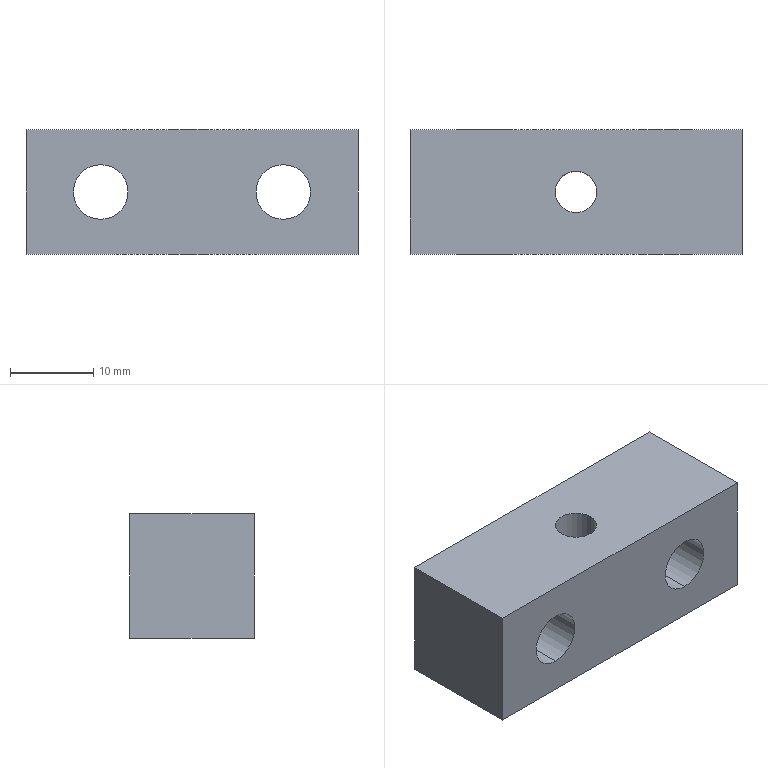Part | STEP file | 0243_214_Block | 1 solid | 12 faces | box 40 x 15 x 15 mm | volume 7679 mm3 | cylinder 6 | plane 6 | commonest cylinder face diameters 6.6 x4 5 x2
STEP:
#1=CARTESIAN_POINT('',(0.,0.,0.));
#2=DIRECTION('',(0.,0.,1.));
#3=DIRECTION('',(1.,0.,0.));
#4=AXIS2_PLACEMENT_3D('',#1,#2,#3);
#5=CARTESIAN_POINT('',(11.,0.,-4.2));
#6=VERTEX_POINT('',#5);
#7=CARTESIAN_POINT('',(11.,15.,-4.2));
#8=VERTEX_POINT('',#7);
#9=CARTESIAN_POINT('',(11.,15.,-4.2));
#10=DIRECTION('',(0.,1.,0.));
#11=VECTOR('',#10,1.);
#12=LINE('',#9,#11);
#13=CARTESIAN_POINT('',(11.,15.,-7.5));
#14=DIRECTION('',(0.,1.,0.));
#15=DIRECTION('',(0.,0.,1.));
#16=AXIS2_PLACEMENT_3D('',#13,#14,#15);
#17=CYLINDRICAL_SURFACE('',#16,3.3);
#18=CARTESIAN_POINT('',(6.283,0.));
#19=DIRECTION('',(0.,1.));
#20=VECTOR('',#19,1.);
#21=LINE('',#18,#20);
#22=(GEOMETRIC_REPRESENTATION_CONTEXT(2)PARAMETRIC_REPRESENTATION_CONTEXT()REPRESENTATION_CONTEXT('',''));
#23=DEFINITIONAL_REPRESENTATION('',(#21),#22);
#24=PCURVE('',#17,#23);
#25=CARTESIAN_POINT('',(11.,15.,-7.5));
#26=DIRECTION('',(0.,1.,0.));
#27=DIRECTION('',(0.,0.,1.));
#28=AXIS2_PLACEMENT_3D('',#25,#26,#27);
#29=CYLINDRICAL_SURFACE('',#28,3.3);
#30=CARTESIAN_POINT('',(0.,0.));
#31=DIRECTION('',(0.,1.));
#32=VECTOR('',#31,1.);
#33=LINE('',#30,#32);
#34=(GEOMETRIC_REPRESENTATION_CONTEXT(2)PARAMETRIC_REPRESENTATION_CONTEXT()REPRESENTATION_CONTEXT('',''));
#35=DEFINITIONAL_REPRESENTATION('',(#33),#34);
#36=PCURVE('',#29,#35);
#37=SURFACE_CURVE('',#12,(#24,#36),.PCURVE_S1.);
#38=EDGE_CURVE('',#6,#8,#37,.T.);
#39=ORIENTED_EDGE('',*,*,#38,.T.);
#40=CARTESIAN_POINT('',(11.,15.,-10.8));
#41=VERTEX_POINT('',#40);
#42=CARTESIAN_POINT('',(11.,15.,-7.5));
#43=DIRECTION('',(0.,1.,0.));
#44=DIRECTION('',(0.,0.,1.));
#45=AXIS2_PLACEMENT_3D('',#42,#43,#44);
#46=CIRCLE('',#45,3.3);
#47=CARTESIAN_POINT('',(0.,0.));
#48=DIRECTION('',(1.,0.));
#49=VECTOR('',#48,1.);
#50=LINE('',#47,#49);
#51=(GEOMETRIC_REPRESENTATION_CONTEXT(2)PARAMETRIC_REPRESENTATION_CONTEXT()REPRESENTATION_CONTEXT('',''));
#52=DEFINITIONAL_REPRESENTATION('',(#50),#51);
#53=PCURVE('',#17,#52);
#54=CARTESIAN_POINT('',(-20.,15.,-15.));
#55=DIRECTION('',(0.,-1.,0.));
#56=DIRECTION('',(0.,0.,-1.));
#57=AXIS2_PLACEMENT_3D('',#54,#55,#56);
#58=PLANE('',#57);
#59=CARTESIAN_POINT('',(-10.8,31.));
#60=CARTESIAN_POINT('',(-10.8,36.716));
#61=CARTESIAN_POINT('',(-5.85,33.858));
#62=CARTESIAN_POINT('',(-0.9,31.));
#63=CARTESIAN_POINT('',(-5.85,28.142));
#64=CARTESIAN_POINT('',(-10.8,25.284));
#65=CARTESIAN_POINT('',(-10.8,31.));
#66=(BOUNDED_CURVE()B_SPLINE_CURVE(2,(#59,#60,#61,#62,#63,#64,#65),.UNSPECIFIED.,.T.,.F.)B_SPLINE_CURVE_WITH_KNOTS((1,2,2,2,2,1),(-2.094,0.,2.094,4.189,6.283,8.378),.UNSPECIFIED.)CURVE()GEOMETRIC_REPRESENTATION_ITEM()RATIONAL_B_SPLINE_CURVE((1.,0.5,1.,0.5,1.,0.5,1.))REPRESENTATION_ITEM(''));
#67=(GEOMETRIC_REPRESENTATION_CONTEXT(2)PARAMETRIC_REPRESENTATION_CONTEXT()REPRESENTATION_CONTEXT('',''));
#68=DEFINITIONAL_REPRESENTATION('',(#66),#67);
#69=PCURVE('',#58,#68);
#70=SURFACE_CURVE('',#46,(#53,#69),.PCURVE_S1.);
#71=EDGE_CURVE('',#41,#8,#70,.T.);
#72=ORIENTED_EDGE('',*,*,#71,.F.);
#73=CARTESIAN_POINT('',(11.,0.,-10.8));
#74=VERTEX_POINT('',#73);
#75=CARTESIAN_POINT('',(11.,15.,-10.8));
#76=DIRECTION('',(0.,1.,0.));
#77=VECTOR('',#76,1.);
#78=LINE('',#75,#77);
#79=CARTESIAN_POINT('',(3.142,0.));
#80=DIRECTION('',(0.,1.));
#81=VECTOR('',#80,1.);
#82=LINE('',#79,#81);
#83=(GEOMETRIC_REPRESENTATION_CONTEXT(2)PARAMETRIC_REPRESENTATION_CONTEXT()REPRESENTATION_CONTEXT('',''));
#84=DEFINITIONAL_REPRESENTATION('',(#82),#83);
#85=PCURVE('',#17,#84);
#86=CARTESIAN_POINT('',(3.142,0.));
#87=DIRECTION('',(0.,1.));
#88=VECTOR('',#87,1.);
#89=LINE('',#86,#88);
#90=(GEOMETRIC_REPRESENTATION_CONTEXT(2)PARAMETRIC_REPRESENTATION_CONTEXT()REPRESENTATION_CONTEXT('',''));
#91=DEFINITIONAL_REPRESENTATION('',(#89),#90);
#92=PCURVE('',#29,#91);
#93=SURFACE_CURVE('',#78,(#85,#92),.PCURVE_S1.);
#94=EDGE_CURVE('',#74,#41,#93,.T.);
#95=ORIENTED_EDGE('',*,*,#94,.F.);
#96=CARTESIAN_POINT('',(11.,0.,-7.5));
#97=DIRECTION('',(0.,1.,0.));
#98=DIRECTION('',(0.,0.,1.));
#99=AXIS2_PLACEMENT_3D('',#96,#97,#98);
#100=CIRCLE('',#99,3.3);
#101=CARTESIAN_POINT('',(0.,-15.));
#102=DIRECTION('',(1.,0.));
#103=VECTOR('',#102,1.);
#104=LINE('',#101,#103);
#105=(GEOMETRIC_REPRESENTATION_CONTEXT(2)PARAMETRIC_REPRESENTATION_CONTEXT()REPRESENTATION_CONTEXT('',''));
#106=DEFINITIONAL_REPRESENTATION('',(#104),#105);
#107=PCURVE('',#17,#106);
#108=CARTESIAN_POINT('',(-20.,0.,-15.));
#109=DIRECTION('',(0.,-1.,0.));
#110=DIRECTION('',(0.,0.,-1.));
#111=AXIS2_PLACEMENT_3D('',#108,#109,#110);
#112=PLANE('',#111);
#113=CARTESIAN_POINT('',(-10.8,31.));
#114=CARTESIAN_POINT('',(-10.8,36.716));
#115=CARTESIAN_POINT('',(-5.85,33.858));
#116=CARTESIAN_POINT('',(-0.9,31.));
#117=CARTESIAN_POINT('',(-5.85,28.142));
#118=CARTESIAN_POINT('',(-10.8,25.284));
#119=CARTESIAN_POINT('',(-10.8,31.));
#120=(BOUNDED_CURVE()B_SPLINE_CURVE(2,(#113,#114,#115,#116,#117,#118,#119),.UNSPECIFIED.,.T.,.F.)B_SPLINE_CURVE_WITH_KNOTS((1,2,2,2,2,1),(-2.094,0.,2.094,4.189,6.283,8.378),.UNSPECIFIED.)CURVE()GEOMETRIC_REPRESENTATION_ITEM()RATIONAL_B_SPLINE_CURVE((1.,0.5,1.,0.5,1.,0.5,1.))REPRESENTATION_ITEM(''));
#121=(GEOMETRIC_REPRESENTATION_CONTEXT(2)PARAMETRIC_REPRESENTATION_CONTEXT()REPRESENTATION_CONTEXT('',''));
#122=DEFINITIONAL_REPRESENTATION('',(#120),#121);
#123=PCURVE('',#112,#122);
#124=SURFACE_CURVE('',#100,(#107,#123),.PCURVE_S1.);
#125=EDGE_CURVE('',#74,#6,#124,.T.);
#126=ORIENTED_EDGE('',*,*,#125,.T.);
#127=EDGE_LOOP('',(#39,#72,#95,#126));
#128=FACE_BOUND('',#127,.F.);
#129=ADVANCED_FACE('',(#128),#17,.F.);
#130=CARTESIAN_POINT('',(-11.,0.,-4.2));
#131=VERTEX_POINT('',#130);
#132=CARTESIAN_POINT('',(-11.,15.,-4.2));
#133=VERTEX_POINT('',#132);
#134=CARTESIAN_POINT('',(-11.,15.,-4.2));
#135=DIRECTION('',(0.,1.,0.));
#136=VECTOR('',#135,1.);
#137=LINE('',#134,#136);
#138=CARTESIAN_POINT('',(-11.,15.,-7.5));
#139=DIRECTION('',(0.,1.,0.));
#140=DIRECTION('',(0.,0.,1.));
#141=AXIS2_PLACEMENT_3D('',#138,#139,#140);
#142=CYLINDRICAL_SURFACE('',#141,3.3);
#143=CARTESIAN_POINT('',(6.283,0.));
#144=DIRECTION('',(0.,1.));
#145=VECTOR('',#144,1.);
#146=LINE('',#143,#145);
#147=(GEOMETRIC_REPRESENTATION_CONTEXT(2)PARAMETRIC_REPRESENTATION_CONTEXT()REPRESENTATION_CONTEXT('',''));
#148=DEFINITIONAL_REPRESENTATION('',(#146),#147);
#149=PCURVE('',#142,#148);
#150=CARTESIAN_POINT('',(-11.,15.,-7.5));
#151=DIRECTION('',(0.,1.,0.));
#152=DIRECTION('',(0.,0.,1.));
#153=AXIS2_PLACEMENT_3D('',#150,#151,#152);
#154=CYLINDRICAL_SURFACE('',#153,3.3);
#155=CARTESIAN_POINT('',(0.,0.));
#156=DIRECTION('',(0.,1.));
#157=VECTOR('',#156,1.);
#158=LINE('',#155,#157);
#159=(GEOMETRIC_REPRESENTATION_CONTEXT(2)PARAMETRIC_REPRESENTATION_CONTEXT()REPRESENTATION_CONTEXT('',''));
#160=DEFINITIONAL_REPRESENTATION('',(#158),#159);
#161=PCURVE('',#154,#160);
#162=SURFACE_CURVE('',#137,(#149,#161),.PCURVE_S1.);
#163=EDGE_CURVE('',#131,#133,#162,.T.);
#164=ORIENTED_EDGE('',*,*,#163,.T.);
#165=CARTESIAN_POINT('',(-11.,15.,-10.8));
#166=VERTEX_POINT('',#165);
#167=CARTESIAN_POINT('',(-11.,15.,-7.5));
#168=DIRECTION('',(0.,1.,0.));
#169=DIRECTION('',(0.,0.,1.));
#170=AXIS2_PLACEMENT_3D('',#167,#168,#169);
#171=CIRCLE('',#170,3.3);
#172=CARTESIAN_POINT('',(0.,0.));
#173=DIRECTION('',(1.,0.));
#174=VECTOR('',#173,1.);
#175=LINE('',#172,#174);
#176=(GEOMETRIC_REPRESENTATION_CONTEXT(2)PARAMETRIC_REPRESENTATION_CONTEXT()REPRESENTATION_CONTEXT('',''));
#177=DEFINITIONAL_REPRESENTATION('',(#175),#176);
#178=PCURVE('',#142,#177);
#179=CARTESIAN_POINT('',(-10.8,9.));
#180=CARTESIAN_POINT('',(-10.8,14.716));
#181=CARTESIAN_POINT('',(-5.85,11.858));
#182=CARTESIAN_POINT('',(-0.9,9.));
#183=CARTESIAN_POINT('',(-5.85,6.142));
#184=CARTESIAN_POINT('',(-10.8,3.284));
#185=CARTESIAN_POINT('',(-10.8,9.));
#186=(BOUNDED_CURVE()B_SPLINE_CURVE(2,(#179,#180,#181,#182,#183,#184,#185),.UNSPECIFIED.,.T.,.F.)B_SPLINE_CURVE_WITH_KNOTS((1,2,2,2,2,1),(-2.094,0.,2.094,4.189,6.283,8.378),.UNSPECIFIED.)CURVE()GEOMETRIC_REPRESENTATION_ITEM()RATIONAL_B_SPLINE_CURVE((1.,0.5,1.,0.5,1.,0.5,1.))REPRESENTATION_ITEM(''));
#187=(GEOMETRIC_REPRESENTATION_CONTEXT(2)PARAMETRIC_REPRESENTATION_CONTEXT()REPRESENTATION_CONTEXT('',''));
#188=DEFINITIONAL_REPRESENTATION('',(#186),#187);
#189=PCURVE('',#58,#188);
#190=SURFACE_CURVE('',#171,(#178,#189),.PCURVE_S1.);
#191=EDGE_CURVE('',#166,#133,#190,.T.);
#192=ORIENTED_EDGE('',*,*,#191,.F.);
#193=CARTESIAN_POINT('',(-11.,0.,-10.8));
#194=VERTEX_POINT('',#193);
#195=CARTESIAN_POINT('',(-11.,15.,-10.8));
#196=DIRECTION('',(0.,1.,0.));
#197=VECTOR('',#196,1.);
#198=LINE('',#195,#197);
#199=CARTESIAN_POINT('',(3.142,0.));
#200=DIRECTION('',(0.,1.));
#201=VECTOR('',#200,1.);
#202=LINE('',#199,#201);
#203=(GEOMETRIC_REPRESENTATION_CONTEXT(2)PARAMETRIC_REPRESENTATION_CONTEXT()REPRESENTATION_CONTEXT('',''));
#204=DEFINITIONAL_REPRESENTATION('',(#202),#203);
#205=PCURVE('',#142,#204);
#206=CARTESIAN_POINT('',(3.142,0.));
#207=DIRECTION('',(0.,1.));
#208=VECTOR('',#207,1.);
#209=LINE('',#206,#208);
#210=(GEOMETRIC_REPRESENTATION_CONTEXT(2)PARAMETRIC_REPRESENTATION_CONTEXT()REPRESENTATION_CONTEXT('',''));
#211=DEFINITIONAL_REPRESENTATION('',(#209),#210);
#212=PCURVE('',#154,#211);
#213=SURFACE_CURVE('',#198,(#205,#212),.PCURVE_S1.);
#214=EDGE_CURVE('',#194,#166,#213,.T.);
#215=ORIENTED_EDGE('',*,*,#214,.F.);
#216=CARTESIAN_POINT('',(-11.,0.,-7.5));
#217=DIRECTION('',(0.,1.,0.));
#218=DIRECTION('',(0.,0.,1.));
#219=AXIS2_PLACEMENT_3D('',#216,#217,#218);
#220=CIRCLE('',#219,3.3);
#221=CARTESIAN_POINT('',(0.,-15.));
#222=DIRECTION('',(1.,0.));
#223=VECTOR('',#222,1.);
#224=LINE('',#221,#223);
#225=(GEOMETRIC_REPRESENTATION_CONTEXT(2)PARAMETRIC_REPRESENTATION_CONTEXT()REPRESENTATION_CONTEXT('',''));
#226=DEFINITIONAL_REPRESENTATION('',(#224),#225);
#227=PCURVE('',#142,#226);
#228=CARTESIAN_POINT('',(-10.8,9.));
#229=CARTESIAN_POINT('',(-10.8,14.716));
#230=CARTESIAN_POINT('',(-5.85,11.858));
#231=CARTESIAN_POINT('',(-0.9,9.));
#232=CARTESIAN_POINT('',(-5.85,6.142));
#233=CARTESIAN_POINT('',(-10.8,3.284));
#234=CARTESIAN_POINT('',(-10.8,9.));
#235=(BOUNDED_CURVE()B_SPLINE_CURVE(2,(#228,#229,#230,#231,#232,#233,#234),.UNSPECIFIED.,.T.,.F.)B_SPLINE_CURVE_WITH_KNOTS((1,2,2,2,2,1),(-2.094,0.,2.094,4.189,6.283,8.378),.UNSPECIFIED.)CURVE()GEOMETRIC_REPRESENTATION_ITEM()RATIONAL_B_SPLINE_CURVE((1.,0.5,1.,0.5,1.,0.5,1.))REPRESENTATION_ITEM(''));
#236=(GEOMETRIC_REPRESENTATION_CONTEXT(2)PARAMETRIC_REPRESENTATION_CONTEXT()REPRESENTATION_CONTEXT('',''));
#237=DEFINITIONAL_REPRESENTATION('',(#235),#236);
#238=PCURVE('',#112,#237);
#239=SURFACE_CURVE('',#220,(#227,#238),.PCURVE_S1.);
#240=EDGE_CURVE('',#194,#131,#239,.T.);
#241=ORIENTED_EDGE('',*,*,#240,.T.);
#242=EDGE_LOOP('',(#164,#192,#215,#241));
#243=FACE_BOUND('',#242,.F.);
#244=ADVANCED_FACE('',(#243),#142,.F.);
#245=CARTESIAN_POINT('',(2.5,7.5,-15.));
#246=VERTEX_POINT('',#245);
#247=CARTESIAN_POINT('',(2.5,7.5,0.));
#248=VERTEX_POINT('',#247);
#249=CARTESIAN_POINT('',(2.5,7.5,0.));
#250=DIRECTION('',(0.,0.,1.));
#251=VECTOR('',#250,1.);
#252=LINE('',#249,#251);
#253=CARTESIAN_POINT('',(0.,7.5,0.));
#254=DIRECTION('',(0.,0.,1.));
#255=DIRECTION('',(1.,0.,0.));
#256=AXIS2_PLACEMENT_3D('',#253,#254,#255);
#257=CYLINDRICAL_SURFACE('',#256,2.5);
#258=CARTESIAN_POINT('',(6.283,0.));
#259=DIRECTION('',(0.,1.));
#260=VECTOR('',#259,1.);
#261=LINE('',#258,#260);
#262=(GEOMETRIC_REPRESENTATION_CONTEXT(2)PARAMETRIC_REPRESENTATION_CONTEXT()REPRESENTATION_CONTEXT('',''));
#263=DEFINITIONAL_REPRESENTATION('',(#261),#262);
#264=PCURVE('',#257,#263);
#265=CARTESIAN_POINT('',(0.,7.5,0.));
#266=DIRECTION('',(0.,0.,1.));
#267=DIRECTION('',(1.,0.,0.));
#268=AXIS2_PLACEMENT_3D('',#265,#266,#267);
#269=CYLINDRICAL_SURFACE('',#268,2.5);
#270=CARTESIAN_POINT('',(0.,0.));
#271=DIRECTION('',(0.,1.));
#272=VECTOR('',#271,1.);
#273=LINE('',#270,#272);
#274=(GEOMETRIC_REPRESENTATION_CONTEXT(2)PARAMETRIC_REPRESENTATION_CONTEXT()REPRESENTATION_CONTEXT('',''));
#275=DEFINITIONAL_REPRESENTATION('',(#273),#274);
#276=PCURVE('',#269,#275);
#277=SURFACE_CURVE('',#252,(#264,#276),.PCURVE_S1.);
#278=EDGE_CURVE('',#246,#248,#277,.T.);
#279=ORIENTED_EDGE('',*,*,#278,.T.);
#280=CARTESIAN_POINT('',(-2.5,7.5,0.));
#281=VERTEX_POINT('',#280);
#282=CARTESIAN_POINT('',(0.,7.5,0.));
#283=DIRECTION('',(0.,0.,1.));
#284=DIRECTION('',(1.,0.,0.));
#285=AXIS2_PLACEMENT_3D('',#282,#283,#284);
#286=CIRCLE('',#285,2.5);
#287=CARTESIAN_POINT('',(0.,0.));
#288=DIRECTION('',(1.,0.));
#289=VECTOR('',#288,1.);
#290=LINE('',#287,#289);
#291=(GEOMETRIC_REPRESENTATION_CONTEXT(2)PARAMETRIC_REPRESENTATION_CONTEXT()REPRESENTATION_CONTEXT('',''));
#292=DEFINITIONAL_REPRESENTATION('',(#290),#291);
#293=PCURVE('',#257,#292);
#294=CARTESIAN_POINT('',(-20.,15.,0.));
#295=DIRECTION('',(0.,0.,-1.));
#296=DIRECTION('',(-1.,0.,0.));
#297=AXIS2_PLACEMENT_3D('',#294,#295,#296);
#298=PLANE('',#297);
#299=CARTESIAN_POINT('',(-22.5,-7.5));
#300=CARTESIAN_POINT('',(-22.5,-3.17));
#301=CARTESIAN_POINT('',(-18.75,-5.335));
#302=CARTESIAN_POINT('',(-15.,-7.5));
#303=CARTESIAN_POINT('',(-18.75,-9.665));
#304=CARTESIAN_POINT('',(-22.5,-11.83));
#305=CARTESIAN_POINT('',(-22.5,-7.5));
#306=(BOUNDED_CURVE()B_SPLINE_CURVE(2,(#299,#300,#301,#302,#303,#304,#305),.UNSPECIFIED.,.T.,.F.)B_SPLINE_CURVE_WITH_KNOTS((1,2,2,2,2,1),(-2.094,0.,2.094,4.189,6.283,8.378),.UNSPECIFIED.)CURVE()GEOMETRIC_REPRESENTATION_ITEM()RATIONAL_B_SPLINE_CURVE((1.,0.5,1.,0.5,1.,0.5,1.))REPRESENTATION_ITEM(''));
#307=(GEOMETRIC_REPRESENTATION_CONTEXT(2)PARAMETRIC_REPRESENTATION_CONTEXT()REPRESENTATION_CONTEXT('',''));
#308=DEFINITIONAL_REPRESENTATION('',(#306),#307);
#309=PCURVE('',#298,#308);
#310=SURFACE_CURVE('',#286,(#293,#309),.PCURVE_S1.);
#311=EDGE_CURVE('',#281,#248,#310,.T.);
#312=ORIENTED_EDGE('',*,*,#311,.F.);
#313=CARTESIAN_POINT('',(-2.5,7.5,-15.));
#314=VERTEX_POINT('',#313);
#315=CARTESIAN_POINT('',(-2.5,7.5,0.));
#316=DIRECTION('',(0.,0.,1.));
#317=VECTOR('',#316,1.);
#318=LINE('',#315,#317);
#319=CARTESIAN_POINT('',(3.142,0.));
#320=DIRECTION('',(0.,1.));
#321=VECTOR('',#320,1.);
#322=LINE('',#319,#321);
#323=(GEOMETRIC_REPRESENTATION_CONTEXT(2)PARAMETRIC_REPRESENTATION_CONTEXT()REPRESENTATION_CONTEXT('',''));
#324=DEFINITIONAL_REPRESENTATION('',(#322),#323);
#325=PCURVE('',#257,#324);
#326=CARTESIAN_POINT('',(3.142,0.));
#327=DIRECTION('',(0.,1.));
#328=VECTOR('',#327,1.);
#329=LINE('',#326,#328);
#330=(GEOMETRIC_REPRESENTATION_CONTEXT(2)PARAMETRIC_REPRESENTATION_CONTEXT()REPRESENTATION_CONTEXT('',''));
#331=DEFINITIONAL_REPRESENTATION('',(#329),#330);
#332=PCURVE('',#269,#331);
#333=SURFACE_CURVE('',#318,(#325,#332),.PCURVE_S1.);
#334=EDGE_CURVE('',#314,#281,#333,.T.);
#335=ORIENTED_EDGE('',*,*,#334,.F.);
#336=CARTESIAN_POINT('',(0.,7.5,-15.));
#337=DIRECTION('',(0.,0.,1.));
#338=DIRECTION('',(1.,0.,0.));
#339=AXIS2_PLACEMENT_3D('',#336,#337,#338);
#340=CIRCLE('',#339,2.5);
#341=CARTESIAN_POINT('',(0.,-15.));
#342=DIRECTION('',(1.,0.));
#343=VECTOR('',#342,1.);
#344=LINE('',#341,#343);
#345=(GEOMETRIC_REPRESENTATION_CONTEXT(2)PARAMETRIC_REPRESENTATION_CONTEXT()REPRESENTATION_CONTEXT('',''));
#346=DEFINITIONAL_REPRESENTATION('',(#344),#345);
#347=PCURVE('',#257,#346);
#348=CARTESIAN_POINT('',(-20.,15.,-15.));
#349=DIRECTION('',(0.,0.,1.));
#350=DIRECTION('',(1.,0.,0.));
#351=AXIS2_PLACEMENT_3D('',#348,#349,#350);
#352=PLANE('',#351);
#353=CARTESIAN_POINT('',(20.,-7.5));
#354=DIRECTION('',(1.,0.));
#355=AXIS2_PLACEMENT_2D('',#353,#354);
#356=CIRCLE('',#355,2.5);
#357=(GEOMETRIC_REPRESENTATION_CONTEXT(2)PARAMETRIC_REPRESENTATION_CONTEXT()REPRESENTATION_CONTEXT('',''));
#358=DEFINITIONAL_REPRESENTATION('',(#356),#357);
#359=PCURVE('',#352,#358);
#360=SURFACE_CURVE('',#340,(#347,#359),.PCURVE_S1.);
#361=EDGE_CURVE('',#314,#246,#360,.T.);
#362=ORIENTED_EDGE('',*,*,#361,.T.);
#363=EDGE_LOOP('',(#279,#312,#335,#362));
#364=FACE_BOUND('',#363,.F.);
#365=ADVANCED_FACE('',(#364),#257,.F.);
#366=CARTESIAN_POINT('',(-20.,0.,-15.));
#367=VERTEX_POINT('',#366);
#368=CARTESIAN_POINT('',(-20.,0.,0.));
#369=VERTEX_POINT('',#368);
#370=CARTESIAN_POINT('',(-20.,0.,0.));
#371=DIRECTION('',(0.,0.,1.));
#372=VECTOR('',#371,1.);
#373=LINE('',#370,#372);
#374=CARTESIAN_POINT('',(-20.,15.,0.));
#375=DIRECTION('',(1.,0.,0.));
#376=DIRECTION('',(0.,0.,-1.));
#377=AXIS2_PLACEMENT_3D('',#374,#375,#376);
#378=PLANE('',#377);
#379=CARTESIAN_POINT('',(0.,-15.));
#380=DIRECTION('',(-1.,0.));
#381=VECTOR('',#380,1.);
#382=LINE('',#379,#381);
#383=(GEOMETRIC_REPRESENTATION_CONTEXT(2)PARAMETRIC_REPRESENTATION_CONTEXT()REPRESENTATION_CONTEXT('',''));
#384=DEFINITIONAL_REPRESENTATION('',(#382),#383);
#385=PCURVE('',#378,#384);
#386=CARTESIAN_POINT('',(-15.,0.));
#387=DIRECTION('',(-1.,0.));
#388=VECTOR('',#387,1.);
#389=LINE('',#386,#388);
#390=(GEOMETRIC_REPRESENTATION_CONTEXT(2)PARAMETRIC_REPRESENTATION_CONTEXT()REPRESENTATION_CONTEXT('',''));
#391=DEFINITIONAL_REPRESENTATION('',(#389),#390);
#392=PCURVE('',#112,#391);
#393=SURFACE_CURVE('',#373,(#385,#392),.PCURVE_S1.);
#394=EDGE_CURVE('',#367,#369,#393,.T.);
#395=ORIENTED_EDGE('',*,*,#394,.T.);
#396=CARTESIAN_POINT('',(-20.,15.,0.));
#397=VERTEX_POINT('',#396);
#398=CARTESIAN_POINT('',(-20.,15.,0.));
#399=DIRECTION('',(0.,-1.,0.));
#400=VECTOR('',#399,1.);
#401=LINE('',#398,#400);
#402=CARTESIAN_POINT('',(0.,0.));
#403=DIRECTION('',(0.,-1.));
#404=VECTOR('',#403,1.);
#405=LINE('',#402,#404);
#406=(GEOMETRIC_REPRESENTATION_CONTEXT(2)PARAMETRIC_REPRESENTATION_CONTEXT()REPRESENTATION_CONTEXT('',''));
#407=DEFINITIONAL_REPRESENTATION('',(#405),#406);
#408=PCURVE('',#378,#407);
#409=CARTESIAN_POINT('',(0.,0.));
#410=DIRECTION('',(0.,-1.));
#411=VECTOR('',#410,1.);
#412=LINE('',#409,#411);
#413=(GEOMETRIC_REPRESENTATION_CONTEXT(2)PARAMETRIC_REPRESENTATION_CONTEXT()REPRESENTATION_CONTEXT('',''));
#414=DEFINITIONAL_REPRESENTATION('',(#412),#413);
#415=PCURVE('',#298,#414);
#416=SURFACE_CURVE('',#401,(#408,#415),.PCURVE_S1.);
#417=EDGE_CURVE('',#397,#369,#416,.T.);
#418=ORIENTED_EDGE('',*,*,#417,.F.);
#419=CARTESIAN_POINT('',(-20.,15.,-15.));
#420=VERTEX_POINT('',#419);
#421=CARTESIAN_POINT('',(-20.,15.,0.));
#422=DIRECTION('',(0.,0.,1.));
#423=VECTOR('',#422,1.);
#424=LINE('',#421,#423);
#425=CARTESIAN_POINT('',(0.,0.));
#426=DIRECTION('',(-1.,0.));
#427=VECTOR('',#426,1.);
#428=LINE('',#425,#427);
#429=(GEOMETRIC_REPRESENTATION_CONTEXT(2)PARAMETRIC_REPRESENTATION_CONTEXT()REPRESENTATION_CONTEXT('',''));
#430=DEFINITIONAL_REPRESENTATION('',(#428),#429);
#431=PCURVE('',#378,#430);
#432=CARTESIAN_POINT('',(-15.,0.));
#433=DIRECTION('',(-1.,0.));
#434=VECTOR('',#433,1.);
#435=LINE('',#432,#434);
#436=(GEOMETRIC_REPRESENTATION_CONTEXT(2)PARAMETRIC_REPRESENTATION_CONTEXT()REPRESENTATION_CONTEXT('',''));
#437=DEFINITIONAL_REPRESENTATION('',(#435),#436);
#438=PCURVE('',#58,#437);
#439=SURFACE_CURVE('',#424,(#431,#438),.PCURVE_S1.);
#440=EDGE_CURVE('',#420,#397,#439,.T.);
#441=ORIENTED_EDGE('',*,*,#440,.F.);
#442=CARTESIAN_POINT('',(-20.,15.,-15.));
#443=DIRECTION('',(0.,-1.,0.));
#444=VECTOR('',#443,1.);
#445=LINE('',#442,#444);
#446=CARTESIAN_POINT('',(15.,0.));
#447=DIRECTION('',(0.,-1.));
#448=VECTOR('',#447,1.);
#449=LINE('',#446,#448);
#450=(GEOMETRIC_REPRESENTATION_CONTEXT(2)PARAMETRIC_REPRESENTATION_CONTEXT()REPRESENTATION_CONTEXT('',''));
#451=DEFINITIONAL_REPRESENTATION('',(#449),#450);
#452=PCURVE('',#378,#451);
#453=CARTESIAN_POINT('',(0.,0.));
#454=DIRECTION('',(0.,-1.));
#455=VECTOR('',#454,1.);
#456=LINE('',#453,#455);
#457=(GEOMETRIC_REPRESENTATION_CONTEXT(2)PARAMETRIC_REPRESENTATION_CONTEXT()REPRESENTATION_CONTEXT('',''));
#458=DEFINITIONAL_REPRESENTATION('',(#456),#457);
#459=PCURVE('',#352,#458);
#460=SURFACE_CURVE('',#445,(#452,#459),.PCURVE_S1.);
#461=EDGE_CURVE('',#420,#367,#460,.T.);
#462=ORIENTED_EDGE('',*,*,#461,.T.);
#463=EDGE_LOOP('',(#395,#418,#441,#462));
#464=FACE_BOUND('',#463,.T.);
#465=ADVANCED_FACE('',(#464),#378,.F.);
#466=CARTESIAN_POINT('',(0.,7.5,0.));
#467=DIRECTION('',(0.,0.,1.));
#468=DIRECTION('',(1.,0.,0.));
#469=AXIS2_PLACEMENT_3D('',#466,#467,#468);
#470=CIRCLE('',#469,2.5);
#471=CARTESIAN_POINT('',(-22.5,-7.5));
#472=CARTESIAN_POINT('',(-22.5,-3.17));
#473=CARTESIAN_POINT('',(-18.75,-5.335));
#474=CARTESIAN_POINT('',(-15.,-7.5));
#475=CARTESIAN_POINT('',(-18.75,-9.665));
#476=CARTESIAN_POINT('',(-22.5,-11.83));
#477=CARTESIAN_POINT('',(-22.5,-7.5));
#478=(BOUNDED_CURVE()B_SPLINE_CURVE(2,(#471,#472,#473,#474,#475,#476,#477),.UNSPECIFIED.,.T.,.F.)B_SPLINE_CURVE_WITH_KNOTS((1,2,2,2,2,1),(-2.094,0.,2.094,4.189,6.283,8.378),.UNSPECIFIED.)CURVE()GEOMETRIC_REPRESENTATION_ITEM()RATIONAL_B_SPLINE_CURVE((1.,0.5,1.,0.5,1.,0.5,1.))REPRESENTATION_ITEM(''));
#479=(GEOMETRIC_REPRESENTATION_CONTEXT(2)PARAMETRIC_REPRESENTATION_CONTEXT()REPRESENTATION_CONTEXT('',''));
#480=DEFINITIONAL_REPRESENTATION('',(#478),#479);
#481=PCURVE('',#298,#480);
#482=CARTESIAN_POINT('',(0.,0.));
#483=DIRECTION('',(1.,0.));
#484=VECTOR('',#483,1.);
#485=LINE('',#482,#484);
#486=(GEOMETRIC_REPRESENTATION_CONTEXT(2)PARAMETRIC_REPRESENTATION_CONTEXT()REPRESENTATION_CONTEXT('',''));
#487=DEFINITIONAL_REPRESENTATION('',(#485),#486);
#488=PCURVE('',#269,#487);
#489=SURFACE_CURVE('',#470,(#481,#488),.PCURVE_S1.);
#490=EDGE_CURVE('',#248,#281,#489,.T.);
#491=ORIENTED_EDGE('',*,*,#490,.F.);
#492=ORIENTED_EDGE('',*,*,#311,.F.);
#493=EDGE_LOOP('',(#491,#492));
#494=FACE_BOUND('',#493,.T.);
#495=CARTESIAN_POINT('',(20.,0.,0.));
#496=VERTEX_POINT('',#495);
#497=CARTESIAN_POINT('',(-20.,0.,0.));
#498=DIRECTION('',(1.,0.,0.));
#499=VECTOR('',#498,1.);
#500=LINE('',#497,#499);
#501=CARTESIAN_POINT('',(0.,-15.));
#502=DIRECTION('',(-1.,0.));
#503=VECTOR('',#502,1.);
#504=LINE('',#501,#503);
#505=(GEOMETRIC_REPRESENTATION_CONTEXT(2)PARAMETRIC_REPRESENTATION_CONTEXT()REPRESENTATION_CONTEXT('',''));
#506=DEFINITIONAL_REPRESENTATION('',(#504),#505);
#507=PCURVE('',#298,#506);
#508=CARTESIAN_POINT('',(-15.,0.));
#509=DIRECTION('',(0.,1.));
#510=VECTOR('',#509,1.);
#511=LINE('',#508,#510);
#512=(GEOMETRIC_REPRESENTATION_CONTEXT(2)PARAMETRIC_REPRESENTATION_CONTEXT()REPRESENTATION_CONTEXT('',''));
#513=DEFINITIONAL_REPRESENTATION('',(#511),#512);
#514=PCURVE('',#112,#513);
#515=SURFACE_CURVE('',#500,(#507,#514),.PCURVE_S1.);
#516=EDGE_CURVE('',#369,#496,#515,.T.);
#517=ORIENTED_EDGE('',*,*,#516,.T.);
#518=CARTESIAN_POINT('',(20.,15.,0.));
#519=VERTEX_POINT('',#518);
#520=CARTESIAN_POINT('',(20.,15.,0.));
#521=DIRECTION('',(0.,-1.,0.));
#522=VECTOR('',#521,1.);
#523=LINE('',#520,#522);
#524=CARTESIAN_POINT('',(-40.,0.));
#525=DIRECTION('',(0.,-1.));
#526=VECTOR('',#525,1.);
#527=LINE('',#524,#526);
#528=(GEOMETRIC_REPRESENTATION_CONTEXT(2)PARAMETRIC_REPRESENTATION_CONTEXT()REPRESENTATION_CONTEXT('',''));
#529=DEFINITIONAL_REPRESENTATION('',(#527),#528);
#530=PCURVE('',#298,#529);
#531=CARTESIAN_POINT('',(20.,15.,0.));
#532=DIRECTION('',(-1.,0.,0.));
#533=DIRECTION('',(0.,0.,1.));
#534=AXIS2_PLACEMENT_3D('',#531,#532,#533);
#535=PLANE('',#534);
#536=CARTESIAN_POINT('',(0.,0.));
#537=DIRECTION('',(0.,-1.));
#538=VECTOR('',#537,1.);
#539=LINE('',#536,#538);
#540=(GEOMETRIC_REPRESENTATION_CONTEXT(2)PARAMETRIC_REPRESENTATION_CONTEXT()REPRESENTATION_CONTEXT('',''));
#541=DEFINITIONAL_REPRESENTATION('',(#539),#540);
#542=PCURVE('',#535,#541);
#543=SURFACE_CURVE('',#523,(#530,#542),.PCURVE_S1.);
#544=EDGE_CURVE('',#519,#496,#543,.T.);
#545=ORIENTED_EDGE('',*,*,#544,.F.);
#546=CARTESIAN_POINT('',(-20.,15.,0.));
#547=DIRECTION('',(1.,0.,0.));
#548=VECTOR('',#547,1.);
#549=LINE('',#546,#548);
#550=CARTESIAN_POINT('',(0.,0.));
#551=DIRECTION('',(-1.,0.));
#552=VECTOR('',#551,1.);
#553=LINE('',#550,#552);
#554=(GEOMETRIC_REPRESENTATION_CONTEXT(2)PARAMETRIC_REPRESENTATION_CONTEXT()REPRESENTATION_CONTEXT('',''));
#555=DEFINITIONAL_REPRESENTATION('',(#553),#554);
#556=PCURVE('',#298,#555);
#557=CARTESIAN_POINT('',(-15.,0.));
#558=DIRECTION('',(0.,1.));
#559=VECTOR('',#558,1.);
#560=LINE('',#557,#559);
#561=(GEOMETRIC_REPRESENTATION_CONTEXT(2)PARAMETRIC_REPRESENTATION_CONTEXT()REPRESENTATION_CONTEXT('',''));
#562=DEFINITIONAL_REPRESENTATION('',(#560),#561);
#563=PCURVE('',#58,#562);
#564=SURFACE_CURVE('',#549,(#556,#563),.PCURVE_S1.);
#565=EDGE_CURVE('',#397,#519,#564,.T.);
#566=ORIENTED_EDGE('',*,*,#565,.F.);
#567=ORIENTED_EDGE('',*,*,#417,.T.);
#568=EDGE_LOOP('',(#517,#545,#566,#567));
#569=FACE_BOUND('',#568,.T.);
#570=ADVANCED_FACE('',(#494,#569),#298,.F.);
#571=CARTESIAN_POINT('',(20.,0.,-15.));
#572=VERTEX_POINT('',#571);
#573=CARTESIAN_POINT('',(20.,0.,0.));
#574=DIRECTION('',(0.,0.,-1.));
#575=VECTOR('',#574,1.);
#576=LINE('',#573,#575);
#577=CARTESIAN_POINT('',(0.,-15.));
#578=DIRECTION('',(-1.,0.));
#579=VECTOR('',#578,1.);
#580=LINE('',#577,#579);
#581=(GEOMETRIC_REPRESENTATION_CONTEXT(2)PARAMETRIC_REPRESENTATION_CONTEXT()REPRESENTATION_CONTEXT('',''));
#582=DEFINITIONAL_REPRESENTATION('',(#580),#581);
#583=PCURVE('',#535,#582);
#584=CARTESIAN_POINT('',(-15.,40.));
#585=DIRECTION('',(1.,0.));
#586=VECTOR('',#585,1.);
#587=LINE('',#584,#586);
#588=(GEOMETRIC_REPRESENTATION_CONTEXT(2)PARAMETRIC_REPRESENTATION_CONTEXT()REPRESENTATION_CONTEXT('',''));
#589=DEFINITIONAL_REPRESENTATION('',(#587),#588);
#590=PCURVE('',#112,#589);
#591=SURFACE_CURVE('',#576,(#583,#590),.PCURVE_S1.);
#592=EDGE_CURVE('',#496,#572,#591,.T.);
#593=ORIENTED_EDGE('',*,*,#592,.T.);
#594=CARTESIAN_POINT('',(20.,15.,-15.));
#595=VERTEX_POINT('',#594);
#596=CARTESIAN_POINT('',(20.,15.,-15.));
#597=DIRECTION('',(0.,-1.,0.));
#598=VECTOR('',#597,1.);
#599=LINE('',#596,#598);
#600=CARTESIAN_POINT('',(-15.,0.));
#601=DIRECTION('',(0.,-1.));
#602=VECTOR('',#601,1.);
#603=LINE('',#600,#602);
#604=(GEOMETRIC_REPRESENTATION_CONTEXT(2)PARAMETRIC_REPRESENTATION_CONTEXT()REPRESENTATION_CONTEXT('',''));
#605=DEFINITIONAL_REPRESENTATION('',(#603),#604);
#606=PCURVE('',#535,#605);
#607=CARTESIAN_POINT('',(40.,0.));
#608=DIRECTION('',(0.,-1.));
#609=VECTOR('',#608,1.);
#610=LINE('',#607,#609);
#611=(GEOMETRIC_REPRESENTATION_CONTEXT(2)PARAMETRIC_REPRESENTATION_CONTEXT()REPRESENTATION_CONTEXT('',''));
#612=DEFINITIONAL_REPRESENTATION('',(#610),#611);
#613=PCURVE('',#352,#612);
#614=SURFACE_CURVE('',#599,(#606,#613),.PCURVE_S1.);
#615=EDGE_CURVE('',#595,#572,#614,.T.);
#616=ORIENTED_EDGE('',*,*,#615,.F.);
#617=CARTESIAN_POINT('',(20.,15.,0.));
#618=DIRECTION('',(0.,0.,-1.));
#619=VECTOR('',#618,1.);
#620=LINE('',#617,#619);
#621=CARTESIAN_POINT('',(0.,0.));
#622=DIRECTION('',(-1.,0.));
#623=VECTOR('',#622,1.);
#624=LINE('',#621,#623);
#625=(GEOMETRIC_REPRESENTATION_CONTEXT(2)PARAMETRIC_REPRESENTATION_CONTEXT()REPRESENTATION_CONTEXT('',''));
#626=DEFINITIONAL_REPRESENTATION('',(#624),#625);
#627=PCURVE('',#535,#626);
#628=CARTESIAN_POINT('',(-15.,40.));
#629=DIRECTION('',(1.,0.));
#630=VECTOR('',#629,1.);
#631=LINE('',#628,#630);
#632=(GEOMETRIC_REPRESENTATION_CONTEXT(2)PARAMETRIC_REPRESENTATION_CONTEXT()REPRESENTATION_CONTEXT('',''));
#633=DEFINITIONAL_REPRESENTATION('',(#631),#632);
#634=PCURVE('',#58,#633);
#635=SURFACE_CURVE('',#620,(#627,#634),.PCURVE_S1.);
#636=EDGE_CURVE('',#519,#595,#635,.T.);
#637=ORIENTED_EDGE('',*,*,#636,.F.);
#638=ORIENTED_EDGE('',*,*,#544,.T.);
#639=EDGE_LOOP('',(#593,#616,#637,#638));
#640=FACE_BOUND('',#639,.T.);
#641=ADVANCED_FACE('',(#640),#535,.F.);
#642=CARTESIAN_POINT('',(0.,7.5,-15.));
#643=DIRECTION('',(0.,0.,1.));
#644=DIRECTION('',(1.,0.,0.));
#645=AXIS2_PLACEMENT_3D('',#642,#643,#644);
#646=CIRCLE('',#645,2.5);
#647=CARTESIAN_POINT('',(20.,-7.5));
#648=DIRECTION('',(1.,0.));
#649=AXIS2_PLACEMENT_2D('',#647,#648);
#650=CIRCLE('',#649,2.5);
#651=(GEOMETRIC_REPRESENTATION_CONTEXT(2)PARAMETRIC_REPRESENTATION_CONTEXT()REPRESENTATION_CONTEXT('',''));
#652=DEFINITIONAL_REPRESENTATION('',(#650),#651);
#653=PCURVE('',#352,#652);
#654=CARTESIAN_POINT('',(0.,-15.));
#655=DIRECTION('',(1.,0.));
#656=VECTOR('',#655,1.);
#657=LINE('',#654,#656);
#658=(GEOMETRIC_REPRESENTATION_CONTEXT(2)PARAMETRIC_REPRESENTATION_CONTEXT()REPRESENTATION_CONTEXT('',''));
#659=DEFINITIONAL_REPRESENTATION('',(#657),#658);
#660=PCURVE('',#269,#659);
#661=SURFACE_CURVE('',#646,(#653,#660),.PCURVE_S1.);
#662=EDGE_CURVE('',#246,#314,#661,.T.);
#663=ORIENTED_EDGE('',*,*,#662,.T.);
#664=ORIENTED_EDGE('',*,*,#361,.T.);
#665=EDGE_LOOP('',(#663,#664));
#666=FACE_BOUND('',#665,.T.);
#667=CARTESIAN_POINT('',(-20.,0.,-15.));
#668=DIRECTION('',(-1.,0.,0.));
#669=VECTOR('',#668,1.);
#670=LINE('',#667,#669);
#671=CARTESIAN_POINT('',(0.,-15.));
#672=DIRECTION('',(-1.,0.));
#673=VECTOR('',#672,1.);
#674=LINE('',#671,#673);
#675=(GEOMETRIC_REPRESENTATION_CONTEXT(2)PARAMETRIC_REPRESENTATION_CONTEXT()REPRESENTATION_CONTEXT('',''));
#676=DEFINITIONAL_REPRESENTATION('',(#674),#675);
#677=PCURVE('',#352,#676);
#678=CARTESIAN_POINT('',(0.,0.));
#679=DIRECTION('',(0.,-1.));
#680=VECTOR('',#679,1.);
#681=LINE('',#678,#680);
#682=(GEOMETRIC_REPRESENTATION_CONTEXT(2)PARAMETRIC_REPRESENTATION_CONTEXT()REPRESENTATION_CONTEXT('',''));
#683=DEFINITIONAL_REPRESENTATION('',(#681),#682);
#684=PCURVE('',#112,#683);
#685=SURFACE_CURVE('',#670,(#677,#684),.PCURVE_S1.);
#686=EDGE_CURVE('',#572,#367,#685,.T.);
#687=ORIENTED_EDGE('',*,*,#686,.T.);
#688=ORIENTED_EDGE('',*,*,#461,.F.);
#689=CARTESIAN_POINT('',(-20.,15.,-15.));
#690=DIRECTION('',(-1.,0.,0.));
#691=VECTOR('',#690,1.);
#692=LINE('',#689,#691);
#693=CARTESIAN_POINT('',(0.,0.));
#694=DIRECTION('',(-1.,0.));
#695=VECTOR('',#694,1.);
#696=LINE('',#693,#695);
#697=(GEOMETRIC_REPRESENTATION_CONTEXT(2)PARAMETRIC_REPRESENTATION_CONTEXT()REPRESENTATION_CONTEXT('',''));
#698=DEFINITIONAL_REPRESENTATION('',(#696),#697);
#699=PCURVE('',#352,#698);
#700=CARTESIAN_POINT('',(0.,0.));
#701=DIRECTION('',(0.,-1.));
#702=VECTOR('',#701,1.);
#703=LINE('',#700,#702);
#704=(GEOMETRIC_REPRESENTATION_CONTEXT(2)PARAMETRIC_REPRESENTATION_CONTEXT()REPRESENTATION_CONTEXT('',''));
#705=DEFINITIONAL_REPRESENTATION('',(#703),#704);
#706=PCURVE('',#58,#705);
#707=SURFACE_CURVE('',#692,(#699,#706),.PCURVE_S1.);
#708=EDGE_CURVE('',#595,#420,#707,.T.);
#709=ORIENTED_EDGE('',*,*,#708,.F.);
#710=ORIENTED_EDGE('',*,*,#615,.T.);
#711=EDGE_LOOP('',(#687,#688,#709,#710));
#712=FACE_BOUND('',#711,.T.);
#713=ADVANCED_FACE('',(#666,#712),#352,.F.);
#714=CARTESIAN_POINT('',(11.,15.,-7.5));
#715=DIRECTION('',(0.,1.,0.));
#716=DIRECTION('',(0.,0.,1.));
#717=AXIS2_PLACEMENT_3D('',#714,#715,#716);
#718=CIRCLE('',#717,3.3);
#719=CARTESIAN_POINT('',(-10.8,31.));
#720=CARTESIAN_POINT('',(-10.8,36.716));
#721=CARTESIAN_POINT('',(-5.85,33.858));
#722=CARTESIAN_POINT('',(-0.9,31.));
#723=CARTESIAN_POINT('',(-5.85,28.142));
#724=CARTESIAN_POINT('',(-10.8,25.284));
#725=CARTESIAN_POINT('',(-10.8,31.));
#726=(BOUNDED_CURVE()B_SPLINE_CURVE(2,(#719,#720,#721,#722,#723,#724,#725),.UNSPECIFIED.,.T.,.F.)B_SPLINE_CURVE_WITH_KNOTS((1,2,2,2,2,1),(-2.094,0.,2.094,4.189,6.283,8.378),.UNSPECIFIED.)CURVE()GEOMETRIC_REPRESENTATION_ITEM()RATIONAL_B_SPLINE_CURVE((1.,0.5,1.,0.5,1.,0.5,1.))REPRESENTATION_ITEM(''));
#727=(GEOMETRIC_REPRESENTATION_CONTEXT(2)PARAMETRIC_REPRESENTATION_CONTEXT()REPRESENTATION_CONTEXT('',''));
#728=DEFINITIONAL_REPRESENTATION('',(#726),#727);
#729=PCURVE('',#58,#728);
#730=CARTESIAN_POINT('',(0.,0.));
#731=DIRECTION('',(1.,0.));
#732=VECTOR('',#731,1.);
#733=LINE('',#730,#732);
#734=(GEOMETRIC_REPRESENTATION_CONTEXT(2)PARAMETRIC_REPRESENTATION_CONTEXT()REPRESENTATION_CONTEXT('',''));
#735=DEFINITIONAL_REPRESENTATION('',(#733),#734);
#736=PCURVE('',#29,#735);
#737=SURFACE_CURVE('',#718,(#729,#736),.PCURVE_S1.);
#738=EDGE_CURVE('',#8,#41,#737,.T.);
#739=ORIENTED_EDGE('',*,*,#738,.F.);
#740=ORIENTED_EDGE('',*,*,#71,.F.);
#741=EDGE_LOOP('',(#739,#740));
#742=FACE_BOUND('',#741,.T.);
#743=CARTESIAN_POINT('',(-11.,15.,-7.5));
#744=DIRECTION('',(0.,1.,0.));
#745=DIRECTION('',(0.,0.,1.));
#746=AXIS2_PLACEMENT_3D('',#743,#744,#745);
#747=CIRCLE('',#746,3.3);
#748=CARTESIAN_POINT('',(-10.8,9.));
#749=CARTESIAN_POINT('',(-10.8,14.716));
#750=CARTESIAN_POINT('',(-5.85,11.858));
#751=CARTESIAN_POINT('',(-0.9,9.));
#752=CARTESIAN_POINT('',(-5.85,6.142));
#753=CARTESIAN_POINT('',(-10.8,3.284));
#754=CARTESIAN_POINT('',(-10.8,9.));
#755=(BOUNDED_CURVE()B_SPLINE_CURVE(2,(#748,#749,#750,#751,#752,#753,#754),.UNSPECIFIED.,.T.,.F.)B_SPLINE_CURVE_WITH_KNOTS((1,2,2,2,2,1),(-2.094,0.,2.094,4.189,6.283,8.378),.UNSPECIFIED.)CURVE()GEOMETRIC_REPRESENTATION_ITEM()RATIONAL_B_SPLINE_CURVE((1.,0.5,1.,0.5,1.,0.5,1.))REPRESENTATION_ITEM(''));
#756=(GEOMETRIC_REPRESENTATION_CONTEXT(2)PARAMETRIC_REPRESENTATION_CONTEXT()REPRESENTATION_CONTEXT('',''));
#757=DEFINITIONAL_REPRESENTATION('',(#755),#756);
#758=PCURVE('',#58,#757);
#759=CARTESIAN_POINT('',(0.,0.));
#760=DIRECTION('',(1.,0.));
#761=VECTOR('',#760,1.);
#762=LINE('',#759,#761);
#763=(GEOMETRIC_REPRESENTATION_CONTEXT(2)PARAMETRIC_REPRESENTATION_CONTEXT()REPRESENTATION_CONTEXT('',''));
#764=DEFINITIONAL_REPRESENTATION('',(#762),#763);
#765=PCURVE('',#154,#764);
#766=SURFACE_CURVE('',#747,(#758,#765),.PCURVE_S1.);
#767=EDGE_CURVE('',#133,#166,#766,.T.);
#768=ORIENTED_EDGE('',*,*,#767,.F.);
#769=ORIENTED_EDGE('',*,*,#191,.F.);
#770=EDGE_LOOP('',(#768,#769));
#771=FACE_BOUND('',#770,.T.);
#772=ORIENTED_EDGE('',*,*,#440,.T.);
#773=ORIENTED_EDGE('',*,*,#565,.T.);
#774=ORIENTED_EDGE('',*,*,#636,.T.);
#775=ORIENTED_EDGE('',*,*,#708,.T.);
#776=EDGE_LOOP('',(#772,#773,#774,#775));
#777=FACE_BOUND('',#776,.T.);
#778=ADVANCED_FACE('',(#742,#771,#777),#58,.F.);
#779=CARTESIAN_POINT('',(11.,0.,-7.5));
#780=DIRECTION('',(0.,1.,0.));
#781=DIRECTION('',(0.,0.,1.));
#782=AXIS2_PLACEMENT_3D('',#779,#780,#781);
#783=CIRCLE('',#782,3.3);
#784=CARTESIAN_POINT('',(-10.8,31.));
#785=CARTESIAN_POINT('',(-10.8,36.716));
#786=CARTESIAN_POINT('',(-5.85,33.858));
#787=CARTESIAN_POINT('',(-0.9,31.));
#788=CARTESIAN_POINT('',(-5.85,28.142));
#789=CARTESIAN_POINT('',(-10.8,25.284));
#790=CARTESIAN_POINT('',(-10.8,31.));
#791=(BOUNDED_CURVE()B_SPLINE_CURVE(2,(#784,#785,#786,#787,#788,#789,#790),.UNSPECIFIED.,.T.,.F.)B_SPLINE_CURVE_WITH_KNOTS((1,2,2,2,2,1),(-2.094,0.,2.094,4.189,6.283,8.378),.UNSPECIFIED.)CURVE()GEOMETRIC_REPRESENTATION_ITEM()RATIONAL_B_SPLINE_CURVE((1.,0.5,1.,0.5,1.,0.5,1.))REPRESENTATION_ITEM(''));
#792=(GEOMETRIC_REPRESENTATION_CONTEXT(2)PARAMETRIC_REPRESENTATION_CONTEXT()REPRESENTATION_CONTEXT('',''));
#793=DEFINITIONAL_REPRESENTATION('',(#791),#792);
#794=PCURVE('',#112,#793);
#795=CARTESIAN_POINT('',(0.,-15.));
#796=DIRECTION('',(1.,0.));
#797=VECTOR('',#796,1.);
#798=LINE('',#795,#797);
#799=(GEOMETRIC_REPRESENTATION_CONTEXT(2)PARAMETRIC_REPRESENTATION_CONTEXT()REPRESENTATION_CONTEXT('',''));
#800=DEFINITIONAL_REPRESENTATION('',(#798),#799);
#801=PCURVE('',#29,#800);
#802=SURFACE_CURVE('',#783,(#794,#801),.PCURVE_S1.);
#803=EDGE_CURVE('',#6,#74,#802,.T.);
#804=ORIENTED_EDGE('',*,*,#803,.T.);
#805=ORIENTED_EDGE('',*,*,#125,.T.);
#806=EDGE_LOOP('',(#804,#805));
#807=FACE_BOUND('',#806,.T.);
#808=CARTESIAN_POINT('',(-11.,0.,-7.5));
#809=DIRECTION('',(0.,1.,0.));
#810=DIRECTION('',(0.,0.,1.));
#811=AXIS2_PLACEMENT_3D('',#808,#809,#810);
#812=CIRCLE('',#811,3.3);
#813=CARTESIAN_POINT('',(-10.8,9.));
#814=CARTESIAN_POINT('',(-10.8,14.716));
#815=CARTESIAN_POINT('',(-5.85,11.858));
#816=CARTESIAN_POINT('',(-0.9,9.));
#817=CARTESIAN_POINT('',(-5.85,6.142));
#818=CARTESIAN_POINT('',(-10.8,3.284));
#819=CARTESIAN_POINT('',(-10.8,9.));
#820=(BOUNDED_CURVE()B_SPLINE_CURVE(2,(#813,#814,#815,#816,#817,#818,#819),.UNSPECIFIED.,.T.,.F.)B_SPLINE_CURVE_WITH_KNOTS((1,2,2,2,2,1),(-2.094,0.,2.094,4.189,6.283,8.378),.UNSPECIFIED.)CURVE()GEOMETRIC_REPRESENTATION_ITEM()RATIONAL_B_SPLINE_CURVE((1.,0.5,1.,0.5,1.,0.5,1.))REPRESENTATION_ITEM(''));
#821=(GEOMETRIC_REPRESENTATION_CONTEXT(2)PARAMETRIC_REPRESENTATION_CONTEXT()REPRESENTATION_CONTEXT('',''));
#822=DEFINITIONAL_REPRESENTATION('',(#820),#821);
#823=PCURVE('',#112,#822);
#824=CARTESIAN_POINT('',(0.,-15.));
#825=DIRECTION('',(1.,0.));
#826=VECTOR('',#825,1.);
#827=LINE('',#824,#826);
#828=(GEOMETRIC_REPRESENTATION_CONTEXT(2)PARAMETRIC_REPRESENTATION_CONTEXT()REPRESENTATION_CONTEXT('',''));
#829=DEFINITIONAL_REPRESENTATION('',(#827),#828);
#830=PCURVE('',#154,#829);
#831=SURFACE_CURVE('',#812,(#823,#830),.PCURVE_S1.);
#832=EDGE_CURVE('',#131,#194,#831,.T.);
#833=ORIENTED_EDGE('',*,*,#832,.T.);
#834=ORIENTED_EDGE('',*,*,#240,.T.);
#835=EDGE_LOOP('',(#833,#834));
#836=FACE_BOUND('',#835,.T.);
#837=ORIENTED_EDGE('',*,*,#394,.F.);
#838=ORIENTED_EDGE('',*,*,#686,.F.);
#839=ORIENTED_EDGE('',*,*,#592,.F.);
#840=ORIENTED_EDGE('',*,*,#516,.F.);
#841=EDGE_LOOP('',(#837,#838,#839,#840));
#842=FACE_BOUND('',#841,.T.);
#843=ADVANCED_FACE('',(#807,#836,#842),#112,.T.);
#844=ORIENTED_EDGE('',*,*,#490,.F.);
#845=ORIENTED_EDGE('',*,*,#278,.F.);
#846=ORIENTED_EDGE('',*,*,#662,.T.);
#847=ORIENTED_EDGE('',*,*,#334,.T.);
#848=EDGE_LOOP('',(#844,#845,#846,#847));
#849=FACE_BOUND('',#848,.F.);
#850=ADVANCED_FACE('',(#849),#269,.F.);
#851=ORIENTED_EDGE('',*,*,#767,.F.);
#852=ORIENTED_EDGE('',*,*,#163,.F.);
#853=ORIENTED_EDGE('',*,*,#832,.T.);
#854=ORIENTED_EDGE('',*,*,#214,.T.);
#855=EDGE_LOOP('',(#851,#852,#853,#854));
#856=FACE_BOUND('',#855,.F.);
#857=ADVANCED_FACE('',(#856),#154,.F.);
#858=ORIENTED_EDGE('',*,*,#738,.F.);
#859=ORIENTED_EDGE('',*,*,#38,.F.);
#860=ORIENTED_EDGE('',*,*,#803,.T.);
#861=ORIENTED_EDGE('',*,*,#94,.T.);
#862=EDGE_LOOP('',(#858,#859,#860,#861));
#863=FACE_BOUND('',#862,.F.);
#864=ADVANCED_FACE('',(#863),#29,.F.);
#865=CLOSED_SHELL('',(#129,#244,#365,#465,#570,#641,#713,#778,#843,#850,#857,#864));
#866=MANIFOLD_SOLID_BREP('',#865);
#867=(LENGTH_UNIT()NAMED_UNIT(*)SI_UNIT(.MILLI.,.METRE.));
#868=UNCERTAINTY_MEASURE_WITH_UNIT(LENGTH_MEASURE(0.0000001),#867,'','');
#869=(NAMED_UNIT(*)PLANE_ANGLE_UNIT()SI_UNIT($,.RADIAN.));
#870=(NAMED_UNIT(*)SI_UNIT($,.STERADIAN.)SOLID_ANGLE_UNIT());
#871=(GEOMETRIC_REPRESENTATION_CONTEXT(3)GLOBAL_UNCERTAINTY_ASSIGNED_CONTEXT((#868))GLOBAL_UNIT_ASSIGNED_CONTEXT((#867,#869,#870))REPRESENTATION_CONTEXT('',''));
#872=ADVANCED_BREP_SHAPE_REPRESENTATION('',(#4,#866),#871);